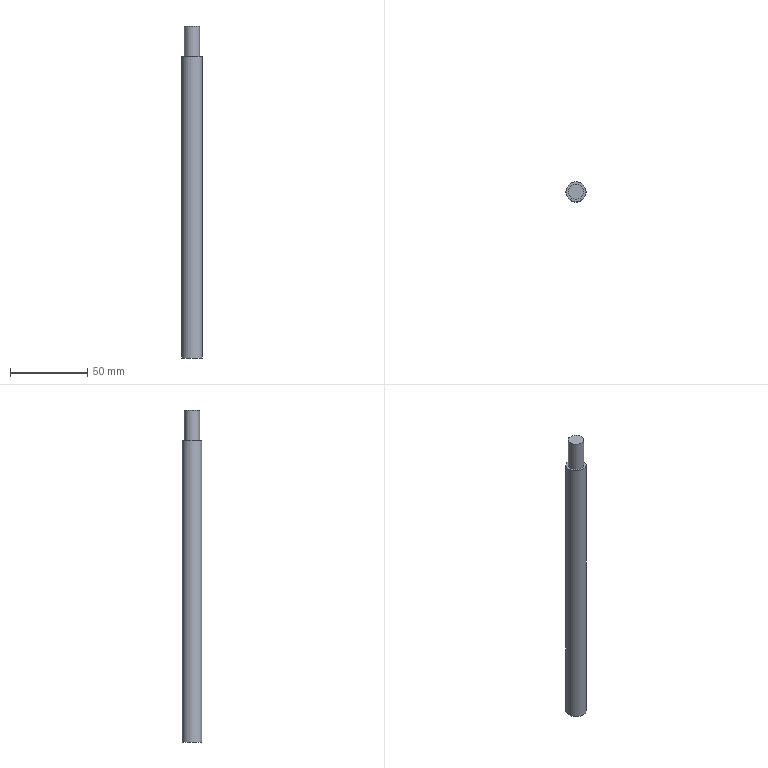Part | NX | features solid 2 | 1 solid | 5 faces | box 13 x 13 x 215 mm | volume 27454 mm3 | plane 3 | cylinder 2 | commonest cylinder face diameters 10 x1 13 x1
STEP:
#1=CARTESIAN_POINT('',(-6.5,727.,-125.));
#2=VERTEX_POINT('',#1);
#3=CARTESIAN_POINT('',(0.,727.,-125.));
#4=DIRECTION('',(0.,0.,-1.));
#5=DIRECTION('',(-1.,0.,0.));
#6=AXIS2_PLACEMENT_3D('',#3,#4,#5);
#7=CIRCLE('',#6,6.5);
#8=EDGE_CURVE('',#2,#2,#7,.F.);
#9=ORIENTED_EDGE('',*,*,#8,.T.);
#10=EDGE_LOOP('',(#9));
#11=FACE_BOUND('',#10,.T.);
#12=CARTESIAN_POINT('',(5.,727.,-125.));
#13=VERTEX_POINT('',#12);
#14=CARTESIAN_POINT('',(0.,727.,-125.));
#15=DIRECTION('',(0.,0.,1.));
#16=DIRECTION('',(1.,0.,0.));
#17=AXIS2_PLACEMENT_3D('',#14,#15,#16);
#18=CIRCLE('',#17,5.);
#19=EDGE_CURVE('',#13,#13,#18,.T.);
#20=ORIENTED_EDGE('',*,*,#19,.F.);
#21=EDGE_LOOP('',(#20));
#22=FACE_BOUND('',#21,.T.);
#23=CARTESIAN_POINT('',(15.,885.,-125.));
#24=DIRECTION('',(0.,0.,-1.));
#25=DIRECTION('',(-1.,0.,0.));
#26=AXIS2_PLACEMENT_3D('',#23,#24,#25);
#27=PLANE('',#26);
#28=ADVANCED_FACE('',(#11,#22),#27,.F.);
#29=ORIENTED_EDGE('',*,*,#8,.F.);
#30=EDGE_LOOP('',(#29));
#31=FACE_BOUND('',#30,.T.);
#32=CARTESIAN_POINT('',(6.5,727.,-320.));
#33=VERTEX_POINT('',#32);
#34=CARTESIAN_POINT('',(0.,727.,-320.));
#35=DIRECTION('',(0.,0.,1.));
#36=DIRECTION('',(1.,0.,0.));
#37=AXIS2_PLACEMENT_3D('',#34,#35,#36);
#38=CIRCLE('',#37,6.5);
#39=EDGE_CURVE('',#33,#33,#38,.T.);
#40=ORIENTED_EDGE('',*,*,#39,.T.);
#41=EDGE_LOOP('',(#40));
#42=FACE_BOUND('',#41,.T.);
#43=CARTESIAN_POINT('',(0.,727.,-1.));
#44=DIRECTION('',(0.,0.,-1.));
#45=DIRECTION('',(-1.,0.,0.));
#46=AXIS2_PLACEMENT_3D('',#43,#44,#45);
#47=CYLINDRICAL_SURFACE('',#46,6.5);
#48=ADVANCED_FACE('',(#31,#42),#47,.T.);
#49=ORIENTED_EDGE('',*,*,#39,.F.);
#50=EDGE_LOOP('',(#49));
#51=FACE_BOUND('',#50,.T.);
#52=CARTESIAN_POINT('',(0.,727.,-320.));
#53=DIRECTION('',(0.,0.,1.));
#54=DIRECTION('',(1.,0.,0.));
#55=AXIS2_PLACEMENT_3D('',#52,#53,#54);
#56=PLANE('',#55);
#57=ADVANCED_FACE('',(#51),#56,.F.);
#58=CARTESIAN_POINT('',(5.,727.,-105.));
#59=VERTEX_POINT('',#58);
#60=CARTESIAN_POINT('',(0.,727.,-105.));
#61=DIRECTION('',(0.,0.,1.));
#62=DIRECTION('',(1.,0.,0.));
#63=AXIS2_PLACEMENT_3D('',#60,#61,#62);
#64=CIRCLE('',#63,5.);
#65=EDGE_CURVE('',#59,#59,#64,.T.);
#66=ORIENTED_EDGE('',*,*,#65,.F.);
#67=EDGE_LOOP('',(#66));
#68=FACE_BOUND('',#67,.T.);
#69=ORIENTED_EDGE('',*,*,#19,.T.);
#70=EDGE_LOOP('',(#69));
#71=FACE_BOUND('',#70,.T.);
#72=CARTESIAN_POINT('',(0.,727.,-105.));
#73=DIRECTION('',(0.,0.,-1.));
#74=DIRECTION('',(-1.,0.,0.));
#75=AXIS2_PLACEMENT_3D('',#72,#73,#74);
#76=CYLINDRICAL_SURFACE('',#75,5.);
#77=ADVANCED_FACE('',(#68,#71),#76,.T.);
#78=ORIENTED_EDGE('',*,*,#65,.T.);
#79=EDGE_LOOP('',(#78));
#80=FACE_BOUND('',#79,.T.);
#81=CARTESIAN_POINT('',(0.,727.,-105.));
#82=DIRECTION('',(0.,0.,1.));
#83=DIRECTION('',(1.,0.,0.));
#84=AXIS2_PLACEMENT_3D('',#81,#82,#83);
#85=PLANE('',#84);
#86=ADVANCED_FACE('',(#80),#85,.T.);
#87=CLOSED_SHELL('',(#28,#48,#57,#77,#86));
#88=MANIFOLD_SOLID_BREP('',#87);
#89=(LENGTH_UNIT()NAMED_UNIT(*)SI_UNIT(.MILLI.,.METRE.));
#90=UNCERTAINTY_MEASURE_WITH_UNIT(LENGTH_MEASURE(0.00001),#89,'','');
#91=(NAMED_UNIT(*)PLANE_ANGLE_UNIT()SI_UNIT($,.RADIAN.));
#92=(NAMED_UNIT(*)SI_UNIT($,.STERADIAN.)SOLID_ANGLE_UNIT());
#93=(GEOMETRIC_REPRESENTATION_CONTEXT(3)GLOBAL_UNCERTAINTY_ASSIGNED_CONTEXT((#90))GLOBAL_UNIT_ASSIGNED_CONTEXT((#89,#91,#92))REPRESENTATION_CONTEXT('',''));
#94=ADVANCED_BREP_SHAPE_REPRESENTATION('',(#88),#93);